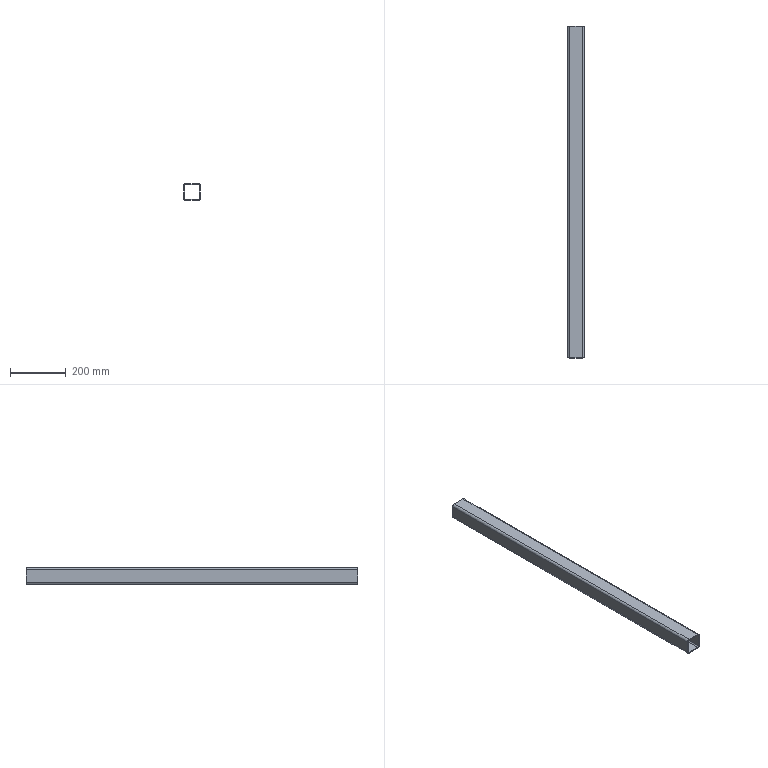Part | SolidWorks | features BaseBody 1 | 1 solid | 18 faces | box 60 x 1190 x 60 mm | volume 1017208 mm3 | plane 10 | cylinder 8 | commonest cylinder face diameters 8 x4 16 x4
STEP:
#1=CARTESIAN_POINT('',(-644.,22.,-1292.));
#2=VERTEX_POINT('',#1);
#3=CARTESIAN_POINT('',(-644.,22.,-1248.));
#4=VERTEX_POINT('',#3);
#5=CARTESIAN_POINT('',(-644.,22.,-1292.));
#6=DIRECTION('',(0.,0.,1.));
#7=VECTOR('',#6,1000.);
#8=LINE('',#5,#7);
#9=EDGE_CURVE('',#2,#4,#8,.T.);
#10=ORIENTED_EDGE('',*,*,#9,.T.);
#11=CARTESIAN_POINT('',(-644.,1212.,-1248.));
#12=VERTEX_POINT('',#11);
#13=CARTESIAN_POINT('',(-644.,1242.,-1248.));
#14=DIRECTION('',(0.,1.,0.));
#15=VECTOR('',#14,1000.);
#16=LINE('',#13,#15);
#17=EDGE_CURVE('',#4,#12,#16,.T.);
#18=ORIENTED_EDGE('',*,*,#17,.T.);
#19=CARTESIAN_POINT('',(-644.,1212.,-1292.));
#20=VERTEX_POINT('',#19);
#21=CARTESIAN_POINT('',(-644.,1212.,-1292.));
#22=DIRECTION('',(0.,0.,-1.));
#23=VECTOR('',#22,1000.);
#24=LINE('',#21,#23);
#25=EDGE_CURVE('',#12,#20,#24,.T.);
#26=ORIENTED_EDGE('',*,*,#25,.T.);
#27=CARTESIAN_POINT('',(-644.,1242.,-1292.));
#28=DIRECTION('',(0.,-1.,0.));
#29=VECTOR('',#28,1000.);
#30=LINE('',#27,#29);
#31=EDGE_CURVE('',#20,#2,#30,.T.);
#32=ORIENTED_EDGE('',*,*,#31,.T.);
#33=EDGE_LOOP('',(#10,#18,#26,#32));
#34=FACE_OUTER_BOUND('',#33,.T.);
#35=CARTESIAN_POINT('',(-644.,1242.,-1292.));
#36=DIRECTION('',(-1.,0.,0.));
#37=DIRECTION('',(0.,0.,1.));
#38=AXIS2_PLACEMENT_3D('',#35,#36,#37);
#39=PLANE('',#38);
#40=ADVANCED_FACE('',(#34),#39,.T.);
#41=ORIENTED_EDGE('',*,*,#17,.F.);
#42=CARTESIAN_POINT('',(-648.,22.,-1244.));
#43=VERTEX_POINT('',#42);
#44=CARTESIAN_POINT('',(-648.,22.,-1248.));
#45=DIRECTION('',(0.,1.,0.));
#46=DIRECTION('',(0.,0.,-1.));
#47=AXIS2_PLACEMENT_3D('',#44,#45,#46);
#48=CIRCLE('',#47,4.);
#49=EDGE_CURVE('',#43,#4,#48,.T.);
#50=ORIENTED_EDGE('',*,*,#49,.F.);
#51=CARTESIAN_POINT('',(-648.,1212.,-1244.));
#52=VERTEX_POINT('',#51);
#53=CARTESIAN_POINT('',(-648.,1242.,-1244.));
#54=DIRECTION('',(0.,-1.,0.));
#55=VECTOR('',#54,1000.);
#56=LINE('',#53,#55);
#57=EDGE_CURVE('',#52,#43,#56,.T.);
#58=ORIENTED_EDGE('',*,*,#57,.F.);
#59=CARTESIAN_POINT('',(-648.,1212.,-1248.));
#60=DIRECTION('',(0.,-1.,0.));
#61=DIRECTION('',(0.,0.,-1.));
#62=AXIS2_PLACEMENT_3D('',#59,#60,#61);
#63=CIRCLE('',#62,4.);
#64=EDGE_CURVE('',#12,#52,#63,.T.);
#65=ORIENTED_EDGE('',*,*,#64,.F.);
#66=EDGE_LOOP('',(#41,#50,#58,#65));
#67=FACE_OUTER_BOUND('',#66,.T.);
#68=CARTESIAN_POINT('',(-648.,1242.,-1248.));
#69=DIRECTION('',(0.,-1.,0.));
#70=DIRECTION('',(0.,0.,-1.));
#71=AXIS2_PLACEMENT_3D('',#68,#69,#70);
#72=CYLINDRICAL_SURFACE('',#71,4.);
#73=ADVANCED_FACE('',(#67),#72,.F.);
#74=CARTESIAN_POINT('',(-648.,22.,-1296.));
#75=VERTEX_POINT('',#74);
#76=CARTESIAN_POINT('',(-648.,22.,-1292.));
#77=DIRECTION('',(0.,-1.,0.));
#78=DIRECTION('',(0.,0.,-1.));
#79=AXIS2_PLACEMENT_3D('',#76,#77,#78);
#80=CIRCLE('',#79,4.);
#81=EDGE_CURVE('',#75,#2,#80,.T.);
#82=ORIENTED_EDGE('',*,*,#81,.F.);
#83=CARTESIAN_POINT('',(-692.,22.,-1296.));
#84=VERTEX_POINT('',#83);
#85=CARTESIAN_POINT('',(-692.,22.,-1296.));
#86=DIRECTION('',(1.,0.,0.));
#87=VECTOR('',#86,1000.);
#88=LINE('',#85,#87);
#89=EDGE_CURVE('',#84,#75,#88,.T.);
#90=ORIENTED_EDGE('',*,*,#89,.F.);
#91=CARTESIAN_POINT('',(-696.,22.,-1292.));
#92=VERTEX_POINT('',#91);
#93=CARTESIAN_POINT('',(-692.,22.,-1292.));
#94=DIRECTION('',(0.,-1.,0.));
#95=DIRECTION('',(0.,0.,-1.));
#96=AXIS2_PLACEMENT_3D('',#93,#94,#95);
#97=CIRCLE('',#96,4.);
#98=EDGE_CURVE('',#92,#84,#97,.T.);
#99=ORIENTED_EDGE('',*,*,#98,.F.);
#100=CARTESIAN_POINT('',(-696.,22.,-1248.));
#101=VERTEX_POINT('',#100);
#102=CARTESIAN_POINT('',(-696.,22.,-1248.));
#103=DIRECTION('',(0.,0.,-1.));
#104=VECTOR('',#103,1000.);
#105=LINE('',#102,#104);
#106=EDGE_CURVE('',#101,#92,#105,.T.);
#107=ORIENTED_EDGE('',*,*,#106,.F.);
#108=CARTESIAN_POINT('',(-692.,22.,-1244.));
#109=VERTEX_POINT('',#108);
#110=CARTESIAN_POINT('',(-692.,22.,-1248.));
#111=DIRECTION('',(0.,-1.,0.));
#112=DIRECTION('',(0.,0.,-1.));
#113=AXIS2_PLACEMENT_3D('',#110,#111,#112);
#114=CIRCLE('',#113,4.);
#115=EDGE_CURVE('',#109,#101,#114,.T.);
#116=ORIENTED_EDGE('',*,*,#115,.F.);
#117=CARTESIAN_POINT('',(-692.,22.,-1244.));
#118=DIRECTION('',(-1.,0.,0.));
#119=VECTOR('',#118,1000.);
#120=LINE('',#117,#119);
#121=EDGE_CURVE('',#43,#109,#120,.T.);
#122=ORIENTED_EDGE('',*,*,#121,.F.);
#123=ORIENTED_EDGE('',*,*,#49,.T.);
#124=ORIENTED_EDGE('',*,*,#9,.F.);
#125=EDGE_LOOP('',(#82,#90,#99,#107,#116,#122,#123,#124));
#126=FACE_BOUND('',#125,.T.);
#127=CARTESIAN_POINT('',(-692.,22.,-1300.));
#128=VERTEX_POINT('',#127);
#129=CARTESIAN_POINT('',(-700.,22.,-1292.));
#130=VERTEX_POINT('',#129);
#131=CARTESIAN_POINT('',(-692.,22.,-1292.));
#132=DIRECTION('',(0.,1.,0.));
#133=DIRECTION('',(0.,0.,-1.));
#134=AXIS2_PLACEMENT_3D('',#131,#132,#133);
#135=CIRCLE('',#134,8.);
#136=EDGE_CURVE('',#128,#130,#135,.T.);
#137=ORIENTED_EDGE('',*,*,#136,.F.);
#138=CARTESIAN_POINT('',(-648.,22.,-1300.));
#139=VERTEX_POINT('',#138);
#140=CARTESIAN_POINT('',(-692.,22.,-1300.));
#141=DIRECTION('',(-1.,0.,0.));
#142=VECTOR('',#141,1000.);
#143=LINE('',#140,#142);
#144=EDGE_CURVE('',#139,#128,#143,.T.);
#145=ORIENTED_EDGE('',*,*,#144,.F.);
#146=CARTESIAN_POINT('',(-640.,22.,-1292.));
#147=VERTEX_POINT('',#146);
#148=CARTESIAN_POINT('',(-648.,22.,-1292.));
#149=DIRECTION('',(0.,1.,0.));
#150=DIRECTION('',(0.,0.,-1.));
#151=AXIS2_PLACEMENT_3D('',#148,#149,#150);
#152=CIRCLE('',#151,8.);
#153=EDGE_CURVE('',#147,#139,#152,.T.);
#154=ORIENTED_EDGE('',*,*,#153,.F.);
#155=CARTESIAN_POINT('',(-640.,22.,-1248.));
#156=VERTEX_POINT('',#155);
#157=CARTESIAN_POINT('',(-640.,22.,-1248.));
#158=DIRECTION('',(0.,0.,-1.));
#159=VECTOR('',#158,1000.);
#160=LINE('',#157,#159);
#161=EDGE_CURVE('',#156,#147,#160,.T.);
#162=ORIENTED_EDGE('',*,*,#161,.F.);
#163=CARTESIAN_POINT('',(-648.,22.,-1240.));
#164=VERTEX_POINT('',#163);
#165=CARTESIAN_POINT('',(-648.,22.,-1248.));
#166=DIRECTION('',(0.,1.,0.));
#167=DIRECTION('',(0.,0.,-1.));
#168=AXIS2_PLACEMENT_3D('',#165,#166,#167);
#169=CIRCLE('',#168,8.);
#170=EDGE_CURVE('',#164,#156,#169,.T.);
#171=ORIENTED_EDGE('',*,*,#170,.F.);
#172=CARTESIAN_POINT('',(-692.,22.,-1240.));
#173=VERTEX_POINT('',#172);
#174=CARTESIAN_POINT('',(-692.,22.,-1240.));
#175=DIRECTION('',(1.,0.,0.));
#176=VECTOR('',#175,1000.);
#177=LINE('',#174,#176);
#178=EDGE_CURVE('',#173,#164,#177,.T.);
#179=ORIENTED_EDGE('',*,*,#178,.F.);
#180=CARTESIAN_POINT('',(-700.,22.,-1248.));
#181=VERTEX_POINT('',#180);
#182=CARTESIAN_POINT('',(-692.,22.,-1248.));
#183=DIRECTION('',(0.,1.,0.));
#184=DIRECTION('',(0.,0.,-1.));
#185=AXIS2_PLACEMENT_3D('',#182,#183,#184);
#186=CIRCLE('',#185,8.);
#187=EDGE_CURVE('',#181,#173,#186,.T.);
#188=ORIENTED_EDGE('',*,*,#187,.F.);
#189=CARTESIAN_POINT('',(-700.,22.,-1248.));
#190=DIRECTION('',(0.,0.,1.));
#191=VECTOR('',#190,1000.);
#192=LINE('',#189,#191);
#193=EDGE_CURVE('',#130,#181,#192,.T.);
#194=ORIENTED_EDGE('',*,*,#193,.F.);
#195=EDGE_LOOP('',(#137,#145,#154,#162,#171,#179,#188,#194));
#196=FACE_OUTER_BOUND('',#195,.T.);
#197=CARTESIAN_POINT('',(-692.,22.,-1248.));
#198=DIRECTION('',(0.,1.,0.));
#199=DIRECTION('',(0.,0.,1.));
#200=AXIS2_PLACEMENT_3D('',#197,#198,#199);
#201=PLANE('',#200);
#202=ADVANCED_FACE('',(#126,#196),#201,.F.);
#203=CARTESIAN_POINT('',(-648.,1212.,-1296.));
#204=VERTEX_POINT('',#203);
#205=CARTESIAN_POINT('',(-648.,1242.,-1296.));
#206=DIRECTION('',(0.,1.,0.));
#207=VECTOR('',#206,1000.);
#208=LINE('',#205,#207);
#209=EDGE_CURVE('',#75,#204,#208,.T.);
#210=ORIENTED_EDGE('',*,*,#209,.F.);
#211=ORIENTED_EDGE('',*,*,#81,.T.);
#212=ORIENTED_EDGE('',*,*,#31,.F.);
#213=CARTESIAN_POINT('',(-648.,1212.,-1292.));
#214=DIRECTION('',(0.,-1.,0.));
#215=DIRECTION('',(0.,0.,-1.));
#216=AXIS2_PLACEMENT_3D('',#213,#214,#215);
#217=CIRCLE('',#216,4.);
#218=EDGE_CURVE('',#204,#20,#217,.T.);
#219=ORIENTED_EDGE('',*,*,#218,.F.);
#220=EDGE_LOOP('',(#210,#211,#212,#219));
#221=FACE_OUTER_BOUND('',#220,.T.);
#222=CARTESIAN_POINT('',(-648.,1242.,-1292.));
#223=DIRECTION('',(0.,-1.,0.));
#224=DIRECTION('',(0.,0.,-1.));
#225=AXIS2_PLACEMENT_3D('',#222,#223,#224);
#226=CYLINDRICAL_SURFACE('',#225,4.);
#227=ADVANCED_FACE('',(#221),#226,.F.);
#228=ORIENTED_EDGE('',*,*,#64,.T.);
#229=CARTESIAN_POINT('',(-692.,1212.,-1244.));
#230=VERTEX_POINT('',#229);
#231=CARTESIAN_POINT('',(-692.,1212.,-1244.));
#232=DIRECTION('',(-1.,0.,0.));
#233=VECTOR('',#232,1000.);
#234=LINE('',#231,#233);
#235=EDGE_CURVE('',#52,#230,#234,.T.);
#236=ORIENTED_EDGE('',*,*,#235,.T.);
#237=CARTESIAN_POINT('',(-696.,1212.,-1248.));
#238=VERTEX_POINT('',#237);
#239=CARTESIAN_POINT('',(-692.,1212.,-1248.));
#240=DIRECTION('',(0.,-1.,0.));
#241=DIRECTION('',(0.,0.,-1.));
#242=AXIS2_PLACEMENT_3D('',#239,#240,#241);
#243=CIRCLE('',#242,4.);
#244=EDGE_CURVE('',#230,#238,#243,.T.);
#245=ORIENTED_EDGE('',*,*,#244,.T.);
#246=CARTESIAN_POINT('',(-696.,1212.,-1292.));
#247=VERTEX_POINT('',#246);
#248=CARTESIAN_POINT('',(-696.,1212.,530.));
#249=DIRECTION('',(0.,0.,-1.));
#250=VECTOR('',#249,1000.);
#251=LINE('',#248,#250);
#252=EDGE_CURVE('',#238,#247,#251,.T.);
#253=ORIENTED_EDGE('',*,*,#252,.T.);
#254=CARTESIAN_POINT('',(-692.,1212.,-1296.));
#255=VERTEX_POINT('',#254);
#256=CARTESIAN_POINT('',(-692.,1212.,-1292.));
#257=DIRECTION('',(0.,-1.,0.));
#258=DIRECTION('',(0.,0.,-1.));
#259=AXIS2_PLACEMENT_3D('',#256,#257,#258);
#260=CIRCLE('',#259,4.);
#261=EDGE_CURVE('',#247,#255,#260,.T.);
#262=ORIENTED_EDGE('',*,*,#261,.T.);
#263=CARTESIAN_POINT('',(-692.,1212.,-1296.));
#264=DIRECTION('',(1.,0.,0.));
#265=VECTOR('',#264,1000.);
#266=LINE('',#263,#265);
#267=EDGE_CURVE('',#255,#204,#266,.T.);
#268=ORIENTED_EDGE('',*,*,#267,.T.);
#269=ORIENTED_EDGE('',*,*,#218,.T.);
#270=ORIENTED_EDGE('',*,*,#25,.F.);
#271=EDGE_LOOP('',(#228,#236,#245,#253,#262,#268,#269,#270));
#272=FACE_BOUND('',#271,.T.);
#273=CARTESIAN_POINT('',(-700.,1212.,-1292.));
#274=VERTEX_POINT('',#273);
#275=CARTESIAN_POINT('',(-700.,1212.,-1248.));
#276=VERTEX_POINT('',#275);
#277=CARTESIAN_POINT('',(-700.,1212.,530.));
#278=DIRECTION('',(0.,0.,1.));
#279=VECTOR('',#278,1000.);
#280=LINE('',#277,#279);
#281=EDGE_CURVE('',#274,#276,#280,.T.);
#282=ORIENTED_EDGE('',*,*,#281,.T.);
#283=CARTESIAN_POINT('',(-692.,1212.,-1240.));
#284=VERTEX_POINT('',#283);
#285=CARTESIAN_POINT('',(-692.,1212.,-1248.));
#286=DIRECTION('',(0.,1.,0.));
#287=DIRECTION('',(0.,0.,-1.));
#288=AXIS2_PLACEMENT_3D('',#285,#286,#287);
#289=CIRCLE('',#288,8.);
#290=EDGE_CURVE('',#276,#284,#289,.T.);
#291=ORIENTED_EDGE('',*,*,#290,.T.);
#292=CARTESIAN_POINT('',(-648.,1212.,-1240.));
#293=VERTEX_POINT('',#292);
#294=CARTESIAN_POINT('',(-692.,1212.,-1240.));
#295=DIRECTION('',(1.,0.,0.));
#296=VECTOR('',#295,1000.);
#297=LINE('',#294,#296);
#298=EDGE_CURVE('',#284,#293,#297,.T.);
#299=ORIENTED_EDGE('',*,*,#298,.T.);
#300=CARTESIAN_POINT('',(-640.,1212.,-1248.));
#301=VERTEX_POINT('',#300);
#302=CARTESIAN_POINT('',(-648.,1212.,-1248.));
#303=DIRECTION('',(0.,1.,0.));
#304=DIRECTION('',(0.,0.,-1.));
#305=AXIS2_PLACEMENT_3D('',#302,#303,#304);
#306=CIRCLE('',#305,8.);
#307=EDGE_CURVE('',#293,#301,#306,.T.);
#308=ORIENTED_EDGE('',*,*,#307,.T.);
#309=CARTESIAN_POINT('',(-640.,1212.,-1292.));
#310=VERTEX_POINT('',#309);
#311=CARTESIAN_POINT('',(-640.,1212.,530.));
#312=DIRECTION('',(0.,0.,-1.));
#313=VECTOR('',#312,1000.);
#314=LINE('',#311,#313);
#315=EDGE_CURVE('',#301,#310,#314,.T.);
#316=ORIENTED_EDGE('',*,*,#315,.T.);
#317=CARTESIAN_POINT('',(-648.,1212.,-1300.));
#318=VERTEX_POINT('',#317);
#319=CARTESIAN_POINT('',(-648.,1212.,-1292.));
#320=DIRECTION('',(0.,1.,0.));
#321=DIRECTION('',(0.,0.,-1.));
#322=AXIS2_PLACEMENT_3D('',#319,#320,#321);
#323=CIRCLE('',#322,8.);
#324=EDGE_CURVE('',#310,#318,#323,.T.);
#325=ORIENTED_EDGE('',*,*,#324,.T.);
#326=CARTESIAN_POINT('',(-692.,1212.,-1300.));
#327=VERTEX_POINT('',#326);
#328=CARTESIAN_POINT('',(-692.,1212.,-1300.));
#329=DIRECTION('',(-1.,0.,0.));
#330=VECTOR('',#329,1000.);
#331=LINE('',#328,#330);
#332=EDGE_CURVE('',#318,#327,#331,.T.);
#333=ORIENTED_EDGE('',*,*,#332,.T.);
#334=CARTESIAN_POINT('',(-692.,1212.,-1292.));
#335=DIRECTION('',(0.,1.,0.));
#336=DIRECTION('',(0.,0.,-1.));
#337=AXIS2_PLACEMENT_3D('',#334,#335,#336);
#338=CIRCLE('',#337,8.);
#339=EDGE_CURVE('',#327,#274,#338,.T.);
#340=ORIENTED_EDGE('',*,*,#339,.T.);
#341=EDGE_LOOP('',(#282,#291,#299,#308,#316,#325,#333,#340));
#342=FACE_OUTER_BOUND('',#341,.T.);
#343=CARTESIAN_POINT('',(-692.,1212.,530.));
#344=DIRECTION('',(0.,1.,0.));
#345=DIRECTION('',(0.,0.,1.));
#346=AXIS2_PLACEMENT_3D('',#343,#344,#345);
#347=PLANE('',#346);
#348=ADVANCED_FACE('',(#272,#342),#347,.T.);
#349=ORIENTED_EDGE('',*,*,#121,.T.);
#350=CARTESIAN_POINT('',(-692.,1242.,-1244.));
#351=DIRECTION('',(0.,1.,0.));
#352=VECTOR('',#351,1000.);
#353=LINE('',#350,#352);
#354=EDGE_CURVE('',#109,#230,#353,.T.);
#355=ORIENTED_EDGE('',*,*,#354,.T.);
#356=ORIENTED_EDGE('',*,*,#235,.F.);
#357=ORIENTED_EDGE('',*,*,#57,.T.);
#358=EDGE_LOOP('',(#349,#355,#356,#357));
#359=FACE_OUTER_BOUND('',#358,.T.);
#360=CARTESIAN_POINT('',(-692.,1242.,-1244.));
#361=DIRECTION('',(0.,0.,-1.));
#362=DIRECTION('',(-1.,0.,0.));
#363=AXIS2_PLACEMENT_3D('',#360,#361,#362);
#364=PLANE('',#363);
#365=ADVANCED_FACE('',(#359),#364,.T.);
#366=ORIENTED_EDGE('',*,*,#89,.T.);
#367=ORIENTED_EDGE('',*,*,#209,.T.);
#368=ORIENTED_EDGE('',*,*,#267,.F.);
#369=CARTESIAN_POINT('',(-692.,1242.,-1296.));
#370=DIRECTION('',(0.,-1.,0.));
#371=VECTOR('',#370,1000.);
#372=LINE('',#369,#371);
#373=EDGE_CURVE('',#255,#84,#372,.T.);
#374=ORIENTED_EDGE('',*,*,#373,.T.);
#375=EDGE_LOOP('',(#366,#367,#368,#374));
#376=FACE_OUTER_BOUND('',#375,.T.);
#377=CARTESIAN_POINT('',(-648.,1242.,-1296.));
#378=DIRECTION('',(0.,0.,1.));
#379=DIRECTION('',(1.,0.,0.));
#380=AXIS2_PLACEMENT_3D('',#377,#378,#379);
#381=PLANE('',#380);
#382=ADVANCED_FACE('',(#376),#381,.T.);
#383=CARTESIAN_POINT('',(-696.,1242.,-1292.));
#384=DIRECTION('',(0.,1.,0.));
#385=VECTOR('',#384,1000.);
#386=LINE('',#383,#385);
#387=EDGE_CURVE('',#92,#247,#386,.T.);
#388=ORIENTED_EDGE('',*,*,#387,.F.);
#389=ORIENTED_EDGE('',*,*,#98,.T.);
#390=ORIENTED_EDGE('',*,*,#373,.F.);
#391=ORIENTED_EDGE('',*,*,#261,.F.);
#392=EDGE_LOOP('',(#388,#389,#390,#391));
#393=FACE_OUTER_BOUND('',#392,.T.);
#394=CARTESIAN_POINT('',(-692.,1242.,-1292.));
#395=DIRECTION('',(0.,-1.,0.));
#396=DIRECTION('',(0.,0.,-1.));
#397=AXIS2_PLACEMENT_3D('',#394,#395,#396);
#398=CYLINDRICAL_SURFACE('',#397,4.);
#399=ADVANCED_FACE('',(#393),#398,.F.);
#400=ORIENTED_EDGE('',*,*,#106,.T.);
#401=ORIENTED_EDGE('',*,*,#387,.T.);
#402=ORIENTED_EDGE('',*,*,#252,.F.);
#403=CARTESIAN_POINT('',(-696.,1242.,-1248.));
#404=DIRECTION('',(0.,-1.,0.));
#405=VECTOR('',#404,1000.);
#406=LINE('',#403,#405);
#407=EDGE_CURVE('',#238,#101,#406,.T.);
#408=ORIENTED_EDGE('',*,*,#407,.T.);
#409=EDGE_LOOP('',(#400,#401,#402,#408));
#410=FACE_OUTER_BOUND('',#409,.T.);
#411=CARTESIAN_POINT('',(-696.,1242.,-1248.));
#412=DIRECTION('',(1.,0.,0.));
#413=DIRECTION('',(0.,0.,-1.));
#414=AXIS2_PLACEMENT_3D('',#411,#412,#413);
#415=PLANE('',#414);
#416=ADVANCED_FACE('',(#410),#415,.T.);
#417=ORIENTED_EDGE('',*,*,#354,.F.);
#418=ORIENTED_EDGE('',*,*,#115,.T.);
#419=ORIENTED_EDGE('',*,*,#407,.F.);
#420=ORIENTED_EDGE('',*,*,#244,.F.);
#421=EDGE_LOOP('',(#417,#418,#419,#420));
#422=FACE_OUTER_BOUND('',#421,.T.);
#423=CARTESIAN_POINT('',(-692.,1242.,-1248.));
#424=DIRECTION('',(0.,-1.,0.));
#425=DIRECTION('',(0.,0.,-1.));
#426=AXIS2_PLACEMENT_3D('',#423,#424,#425);
#427=CYLINDRICAL_SURFACE('',#426,4.);
#428=ADVANCED_FACE('',(#422),#427,.F.);
#429=ORIENTED_EDGE('',*,*,#193,.T.);
#430=CARTESIAN_POINT('',(-700.,1242.,-1248.));
#431=DIRECTION('',(0.,-1.,0.));
#432=VECTOR('',#431,1000.);
#433=LINE('',#430,#432);
#434=EDGE_CURVE('',#276,#181,#433,.T.);
#435=ORIENTED_EDGE('',*,*,#434,.F.);
#436=ORIENTED_EDGE('',*,*,#281,.F.);
#437=CARTESIAN_POINT('',(-700.,1242.,-1292.));
#438=DIRECTION('',(0.,1.,0.));
#439=VECTOR('',#438,1000.);
#440=LINE('',#437,#439);
#441=EDGE_CURVE('',#130,#274,#440,.T.);
#442=ORIENTED_EDGE('',*,*,#441,.F.);
#443=EDGE_LOOP('',(#429,#435,#436,#442));
#444=FACE_OUTER_BOUND('',#443,.T.);
#445=CARTESIAN_POINT('',(-700.,1242.,-1248.));
#446=DIRECTION('',(1.,0.,0.));
#447=DIRECTION('',(0.,0.,-1.));
#448=AXIS2_PLACEMENT_3D('',#445,#446,#447);
#449=PLANE('',#448);
#450=ADVANCED_FACE('',(#444),#449,.F.);
#451=ORIENTED_EDGE('',*,*,#441,.T.);
#452=ORIENTED_EDGE('',*,*,#339,.F.);
#453=CARTESIAN_POINT('',(-692.,1242.,-1300.));
#454=DIRECTION('',(0.,-1.,0.));
#455=VECTOR('',#454,1000.);
#456=LINE('',#453,#455);
#457=EDGE_CURVE('',#327,#128,#456,.T.);
#458=ORIENTED_EDGE('',*,*,#457,.T.);
#459=ORIENTED_EDGE('',*,*,#136,.T.);
#460=EDGE_LOOP('',(#451,#452,#458,#459));
#461=FACE_OUTER_BOUND('',#460,.T.);
#462=CARTESIAN_POINT('',(-692.,1242.,-1292.));
#463=DIRECTION('',(0.,-1.,0.));
#464=DIRECTION('',(0.,0.,-1.));
#465=AXIS2_PLACEMENT_3D('',#462,#463,#464);
#466=CYLINDRICAL_SURFACE('',#465,8.);
#467=ADVANCED_FACE('',(#461),#466,.T.);
#468=ORIENTED_EDGE('',*,*,#144,.T.);
#469=ORIENTED_EDGE('',*,*,#457,.F.);
#470=ORIENTED_EDGE('',*,*,#332,.F.);
#471=CARTESIAN_POINT('',(-648.,1242.,-1300.));
#472=DIRECTION('',(0.,1.,0.));
#473=VECTOR('',#472,1000.);
#474=LINE('',#471,#473);
#475=EDGE_CURVE('',#139,#318,#474,.T.);
#476=ORIENTED_EDGE('',*,*,#475,.F.);
#477=EDGE_LOOP('',(#468,#469,#470,#476));
#478=FACE_OUTER_BOUND('',#477,.T.);
#479=CARTESIAN_POINT('',(-648.,1242.,-1300.));
#480=DIRECTION('',(0.,0.,1.));
#481=DIRECTION('',(1.,0.,0.));
#482=AXIS2_PLACEMENT_3D('',#479,#480,#481);
#483=PLANE('',#482);
#484=ADVANCED_FACE('',(#478),#483,.F.);
#485=ORIENTED_EDGE('',*,*,#475,.T.);
#486=ORIENTED_EDGE('',*,*,#324,.F.);
#487=CARTESIAN_POINT('',(-640.,1242.,-1292.));
#488=DIRECTION('',(0.,-1.,0.));
#489=VECTOR('',#488,1000.);
#490=LINE('',#487,#489);
#491=EDGE_CURVE('',#310,#147,#490,.T.);
#492=ORIENTED_EDGE('',*,*,#491,.T.);
#493=ORIENTED_EDGE('',*,*,#153,.T.);
#494=EDGE_LOOP('',(#485,#486,#492,#493));
#495=FACE_OUTER_BOUND('',#494,.T.);
#496=CARTESIAN_POINT('',(-648.,1242.,-1292.));
#497=DIRECTION('',(0.,-1.,0.));
#498=DIRECTION('',(0.,0.,-1.));
#499=AXIS2_PLACEMENT_3D('',#496,#497,#498);
#500=CYLINDRICAL_SURFACE('',#499,8.);
#501=ADVANCED_FACE('',(#495),#500,.T.);
#502=ORIENTED_EDGE('',*,*,#161,.T.);
#503=ORIENTED_EDGE('',*,*,#491,.F.);
#504=ORIENTED_EDGE('',*,*,#315,.F.);
#505=CARTESIAN_POINT('',(-640.,1242.,-1248.));
#506=DIRECTION('',(0.,1.,0.));
#507=VECTOR('',#506,1000.);
#508=LINE('',#505,#507);
#509=EDGE_CURVE('',#156,#301,#508,.T.);
#510=ORIENTED_EDGE('',*,*,#509,.F.);
#511=EDGE_LOOP('',(#502,#503,#504,#510));
#512=FACE_OUTER_BOUND('',#511,.T.);
#513=CARTESIAN_POINT('',(-640.,1242.,-1292.));
#514=DIRECTION('',(-1.,0.,0.));
#515=DIRECTION('',(0.,0.,1.));
#516=AXIS2_PLACEMENT_3D('',#513,#514,#515);
#517=PLANE('',#516);
#518=ADVANCED_FACE('',(#512),#517,.F.);
#519=ORIENTED_EDGE('',*,*,#509,.T.);
#520=ORIENTED_EDGE('',*,*,#307,.F.);
#521=CARTESIAN_POINT('',(-648.,1242.,-1240.));
#522=DIRECTION('',(0.,-1.,0.));
#523=VECTOR('',#522,1000.);
#524=LINE('',#521,#523);
#525=EDGE_CURVE('',#293,#164,#524,.T.);
#526=ORIENTED_EDGE('',*,*,#525,.T.);
#527=ORIENTED_EDGE('',*,*,#170,.T.);
#528=EDGE_LOOP('',(#519,#520,#526,#527));
#529=FACE_OUTER_BOUND('',#528,.T.);
#530=CARTESIAN_POINT('',(-648.,1242.,-1248.));
#531=DIRECTION('',(0.,-1.,0.));
#532=DIRECTION('',(0.,0.,-1.));
#533=AXIS2_PLACEMENT_3D('',#530,#531,#532);
#534=CYLINDRICAL_SURFACE('',#533,8.);
#535=ADVANCED_FACE('',(#529),#534,.T.);
#536=ORIENTED_EDGE('',*,*,#178,.T.);
#537=ORIENTED_EDGE('',*,*,#525,.F.);
#538=ORIENTED_EDGE('',*,*,#298,.F.);
#539=CARTESIAN_POINT('',(-692.,1242.,-1240.));
#540=DIRECTION('',(0.,1.,0.));
#541=VECTOR('',#540,1000.);
#542=LINE('',#539,#541);
#543=EDGE_CURVE('',#173,#284,#542,.T.);
#544=ORIENTED_EDGE('',*,*,#543,.F.);
#545=EDGE_LOOP('',(#536,#537,#538,#544));
#546=FACE_OUTER_BOUND('',#545,.T.);
#547=CARTESIAN_POINT('',(-692.,1242.,-1240.));
#548=DIRECTION('',(0.,0.,-1.));
#549=DIRECTION('',(-1.,0.,0.));
#550=AXIS2_PLACEMENT_3D('',#547,#548,#549);
#551=PLANE('',#550);
#552=ADVANCED_FACE('',(#546),#551,.F.);
#553=ORIENTED_EDGE('',*,*,#543,.T.);
#554=ORIENTED_EDGE('',*,*,#290,.F.);
#555=ORIENTED_EDGE('',*,*,#434,.T.);
#556=ORIENTED_EDGE('',*,*,#187,.T.);
#557=EDGE_LOOP('',(#553,#554,#555,#556));
#558=FACE_OUTER_BOUND('',#557,.T.);
#559=CARTESIAN_POINT('',(-692.,1242.,-1248.));
#560=DIRECTION('',(0.,-1.,0.));
#561=DIRECTION('',(0.,0.,-1.));
#562=AXIS2_PLACEMENT_3D('',#559,#560,#561);
#563=CYLINDRICAL_SURFACE('',#562,8.);
#564=ADVANCED_FACE('',(#558),#563,.T.);
#565=CLOSED_SHELL('',(#40,#73,#202,#227,#348,#365,#382,#399,#416,#428,#450,#467,#484,#501,#518,#535,#552,#564));
#566=MANIFOLD_SOLID_BREP('',#565);
#567=CARTESIAN_POINT('',(0.,0.,0.));
#568=DIRECTION('',(0.,0.,1.));
#569=DIRECTION('',(1.,0.,0.));
#570=AXIS2_PLACEMENT_3D('',#567,#568,#569);
#571=(LENGTH_UNIT()NAMED_UNIT(*)SI_UNIT(.MILLI.,.METRE.));
#572=UNCERTAINTY_MEASURE_WITH_UNIT(LENGTH_MEASURE(0.00001),#571,'','');
#573=(NAMED_UNIT(*)PLANE_ANGLE_UNIT()SI_UNIT($,.RADIAN.));
#574=(NAMED_UNIT(*)SI_UNIT($,.STERADIAN.)SOLID_ANGLE_UNIT());
#575=(GEOMETRIC_REPRESENTATION_CONTEXT(3)GLOBAL_UNCERTAINTY_ASSIGNED_CONTEXT((#572))GLOBAL_UNIT_ASSIGNED_CONTEXT((#571,#573,#574))REPRESENTATION_CONTEXT('',''));
#576=ADVANCED_BREP_SHAPE_REPRESENTATION('',(#566,#570),#575);